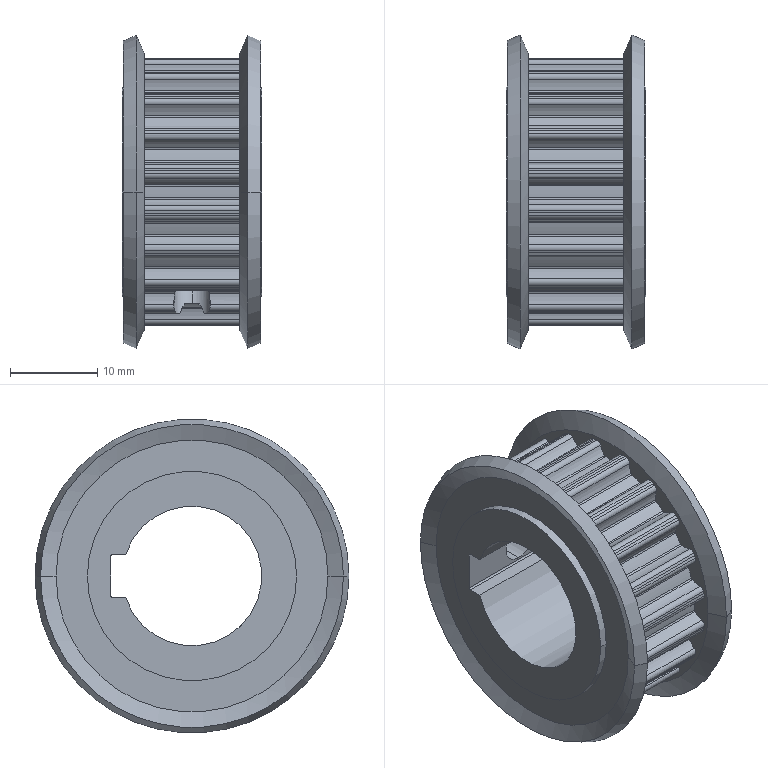Part | NX | 1 solid | 224 faces | box 16 x 36 x 36 mm | volume 7721 mm3 | cylinder 203 | cone 12 | plane 9 | commonest cylinder face diameters 6.55 x44 0.5 x43 1.1 x42 30.87 x42 27.33 x21 4.134 x4